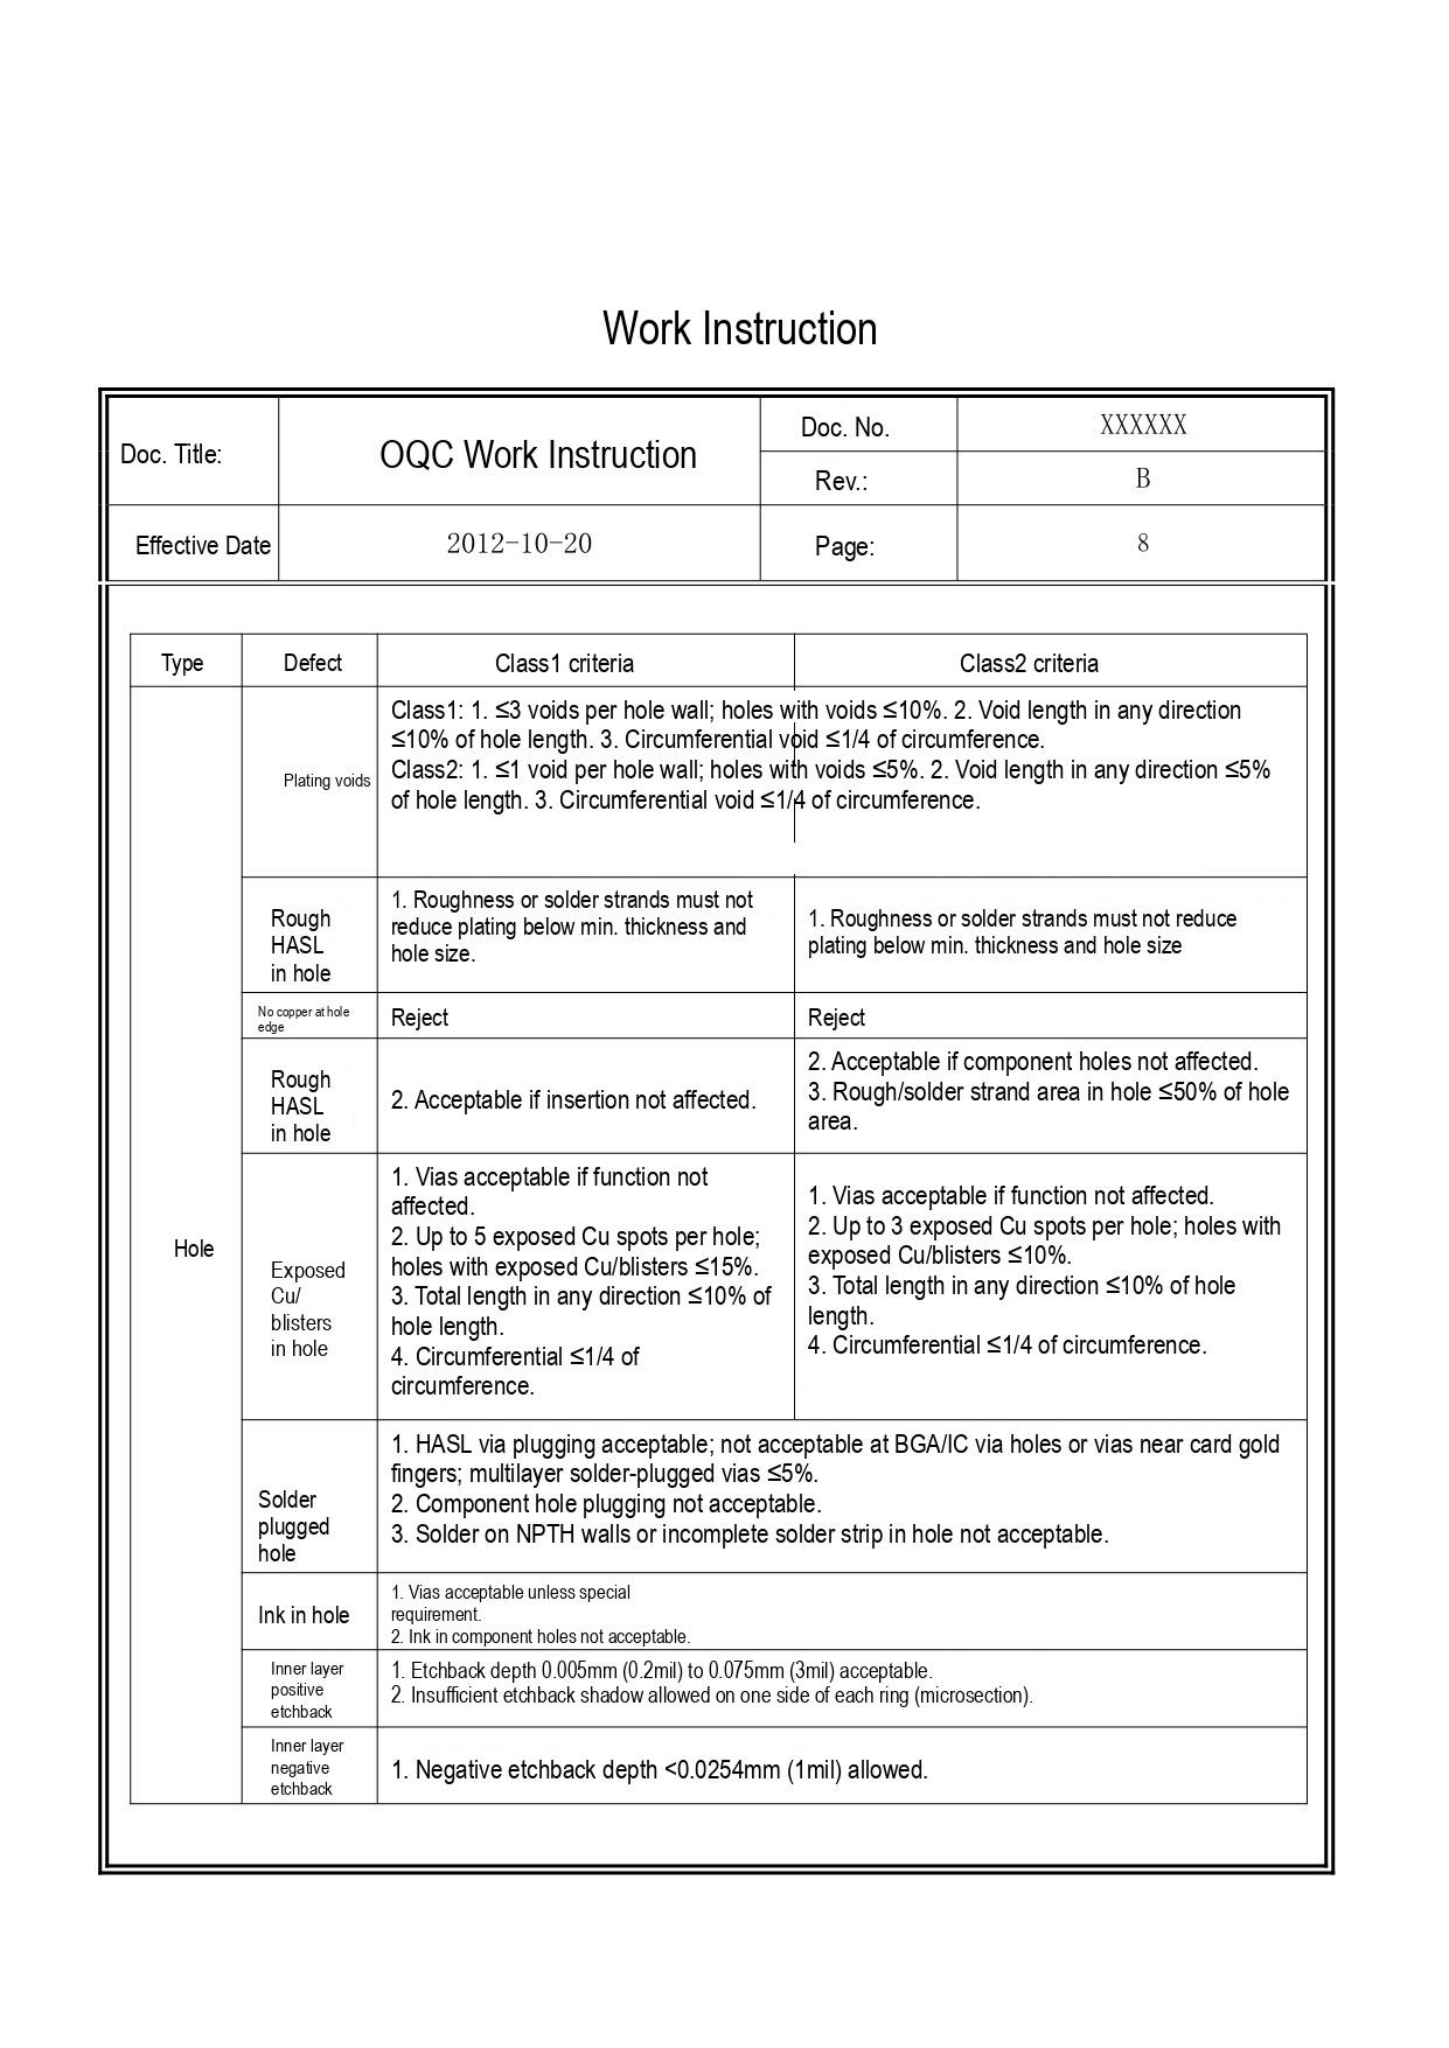# Work Instruction

| Doc. Title: | OQC Work Instruction | Doc. No. | XXXXXX |
|---|---|---|---|
| | | Rev.: | B |
| Effective Date | 2012-10-20 | Page: | 8 |

| Type | Defect | Class1 criteria | Class2 criteria |
|---|---|---|---|
| Hole | Plating voids | Class1: 1. ≤3 voids per hole wall; holes with voids ≤10%. 2. Void length in any direction ≤10% of hole length. 3. Circumferential void ≤1/4 of circumference.<br>Class2: 1. ≤1 void per hole wall; holes with voids ≤5%. 2. Void length in any direction ≤5% of hole length. 3. Circumferential void ≤1/4 of circumference. | |
| | Rough HASL in hole | 1. Roughness or solder strands must not reduce plating below min. thickness and hole size. | 1. Roughness or solder strands must not reduce plating below min. thickness and hole size |
| | No copper at hole edge | Reject | Reject |
| | Rough HASL in hole | 2. Acceptable if insertion not affected. | 2. Acceptable if component holes not affected.<br>3. Rough/solder strand area in hole ≤50% of hole area. |
| | Exposed Cu/ blisters in hole | 1. Vias acceptable if function not affected.<br>2. Up to 5 exposed Cu spots per hole; holes with exposed Cu/blisters ≤15%.<br>3. Total length in any direction ≤10% of hole length.<br>4. Circumferential ≤1/4 of circumference. | 1. Vias acceptable if function not affected.<br>2. Up to 3 exposed Cu spots per hole; holes with exposed Cu/blisters ≤10%.<br>3. Total length in any direction ≤10% of hole length.<br>4. Circumferential ≤1/4 of circumference. |
| | Solder plugged hole | 1. HASL via plugging acceptable; not acceptable at BGA/IC via holes or vias near card gold fingers; multilayer solder-plugged vias ≤5%.<br>2. Component hole plugging not acceptable.<br>3. Solder on NPTH walls or incomplete solder strip in hole not acceptable. | |
| | Ink in hole | 1. Vias acceptable unless special requirement.<br>2. Ink in component holes not acceptable. | |
| | Inner layer positive etchback | 1. Etchback depth 0.005mm (0.2mil) to 0.075mm (3mil) acceptable.<br>2. Insufficient etchback shadow allowed on one side of each ring (microsection). | |
| | Inner layer negative etchback | 1. Negative etchback depth <0.0254mm (1mil) allowed. | |
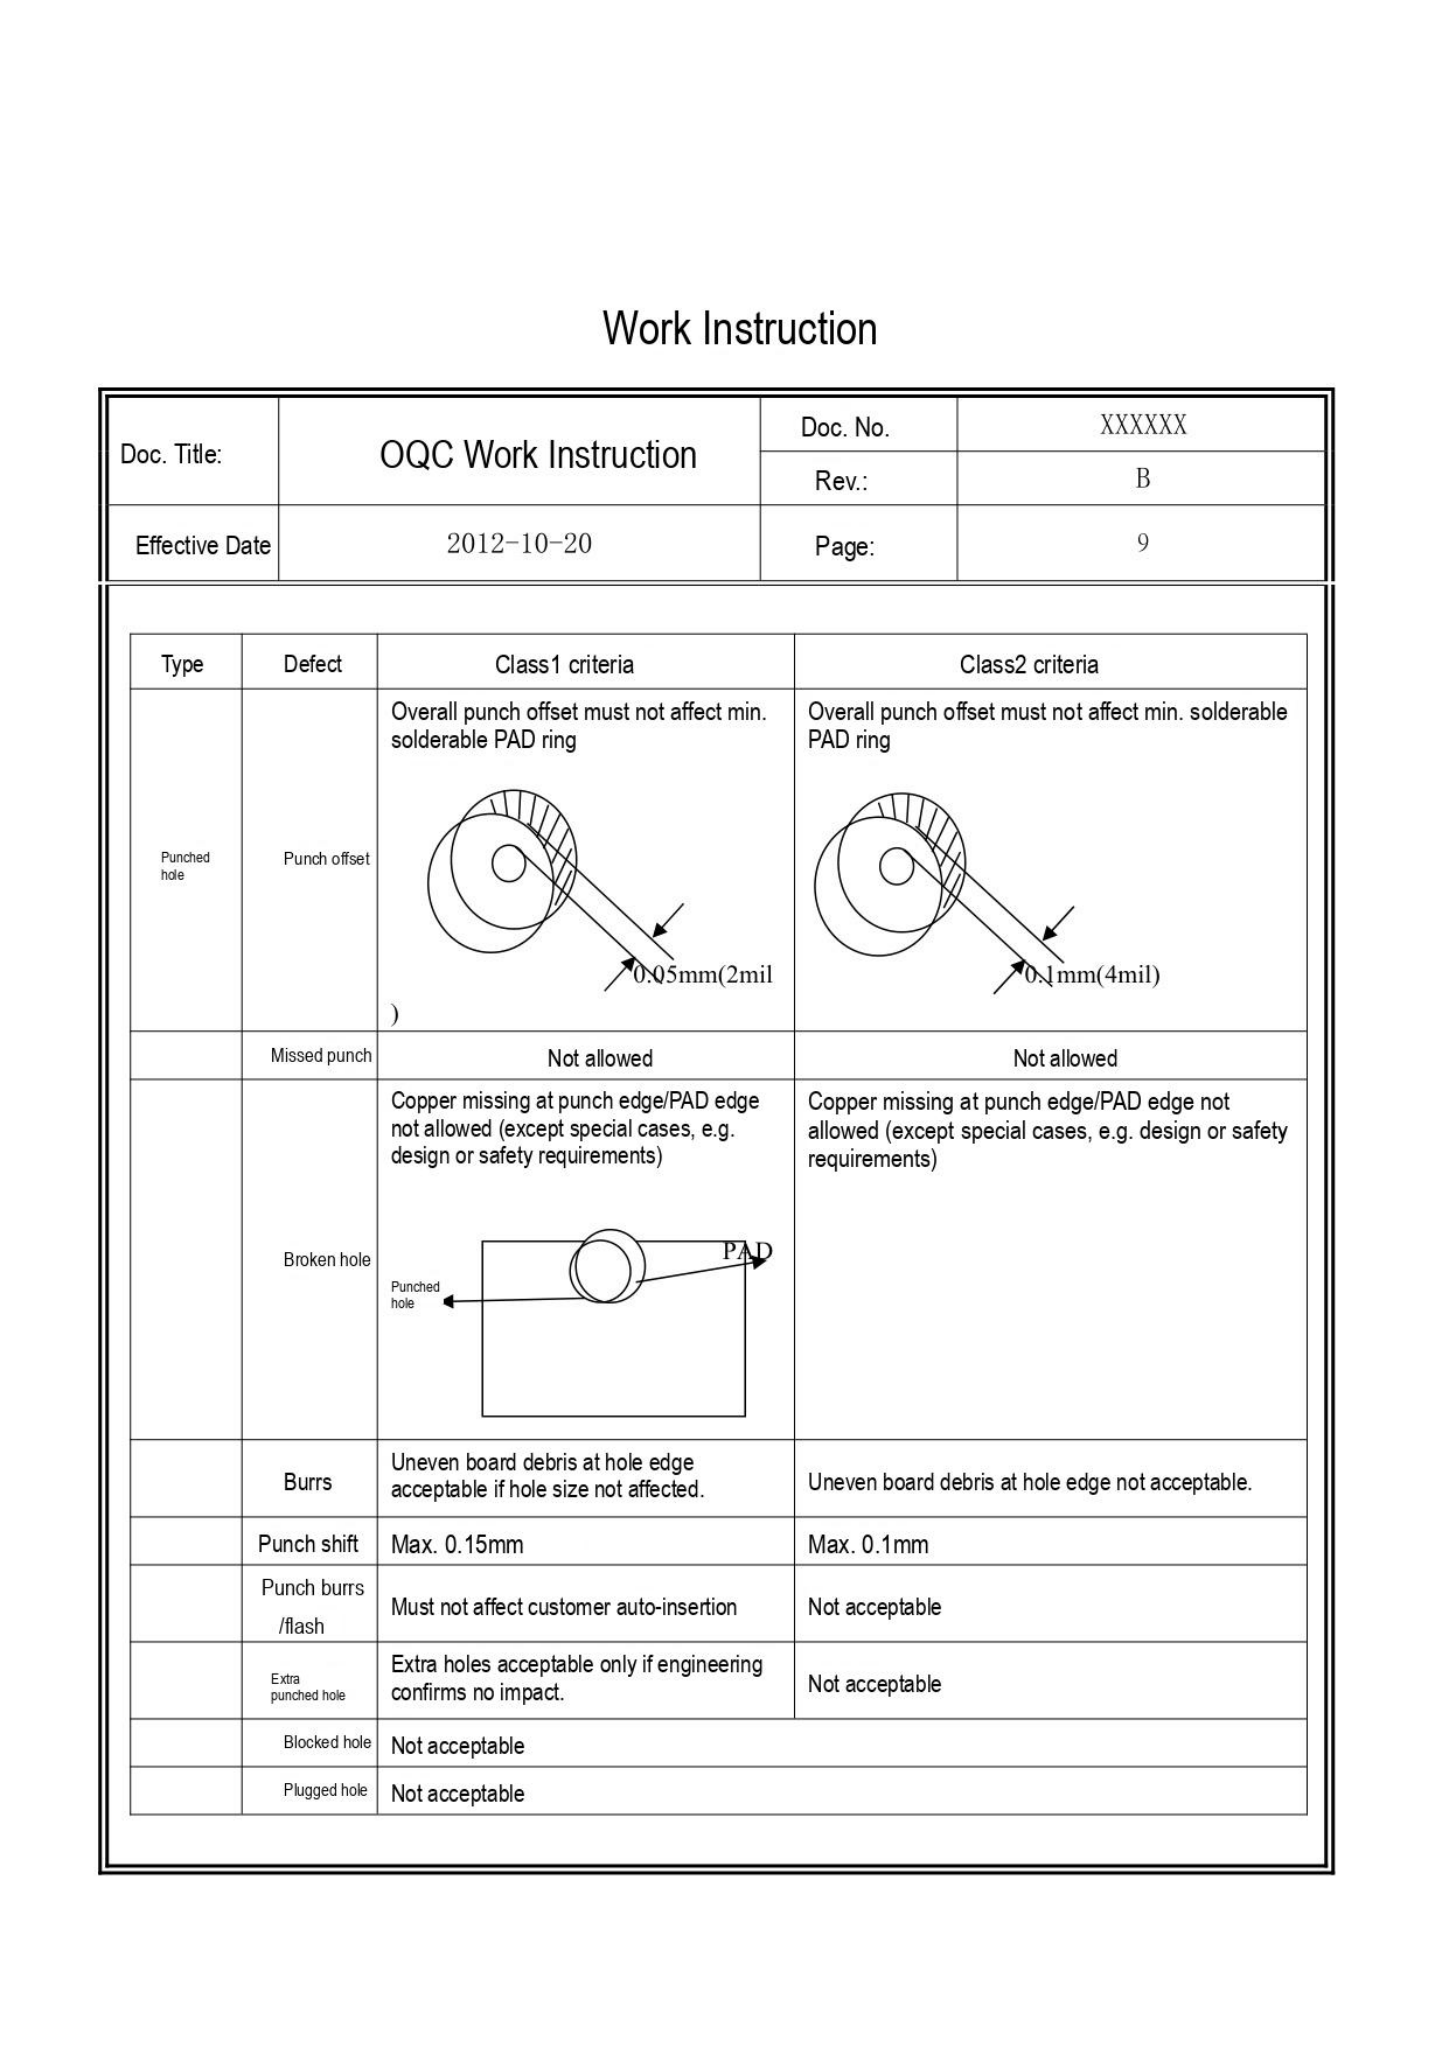Work Instruction

| Doc. Title: | OQC Work Instruction | Doc. No. | XXXXXX |
|---|---|---|---|
| | | Rev.: | B |
| Effective Date | 2012-10-20 | Page: | 9 |

| Type | Defect | Class1 criteria | Class2 criteria |
|---|---|---|---|
| Punched hole | Punch offset | Overall punch offset must not affect min. solderable PAD ring<br>0.05mm(2mil<br>) | Overall punch offset must not affect min. solderable PAD ring<br>0.1mm(4mil) |
| | Missed punch | Not allowed | Not allowed |
| | Broken hole | Copper missing at punch edge/PAD edge not allowed (except special cases, e.g. design or safety requirements)<br>PAD<br>Punched hole | Copper missing at punch edge/PAD edge not allowed (except special cases, e.g. design or safety requirements) |
| | Burrs | Uneven board debris at hole edge acceptable if hole size not affected. | Uneven board debris at hole edge not acceptable. |
| | Punch shift | Max. 0.15mm | Max. 0.1mm |
| | Punch burrs /flash | Must not affect customer auto-insertion | Not acceptable |
| | Extra punched hole | Extra holes acceptable only if engineering confirms no impact. | Not acceptable |
| | Blocked hole | Not acceptable | |
| | Plugged hole | Not acceptable | |
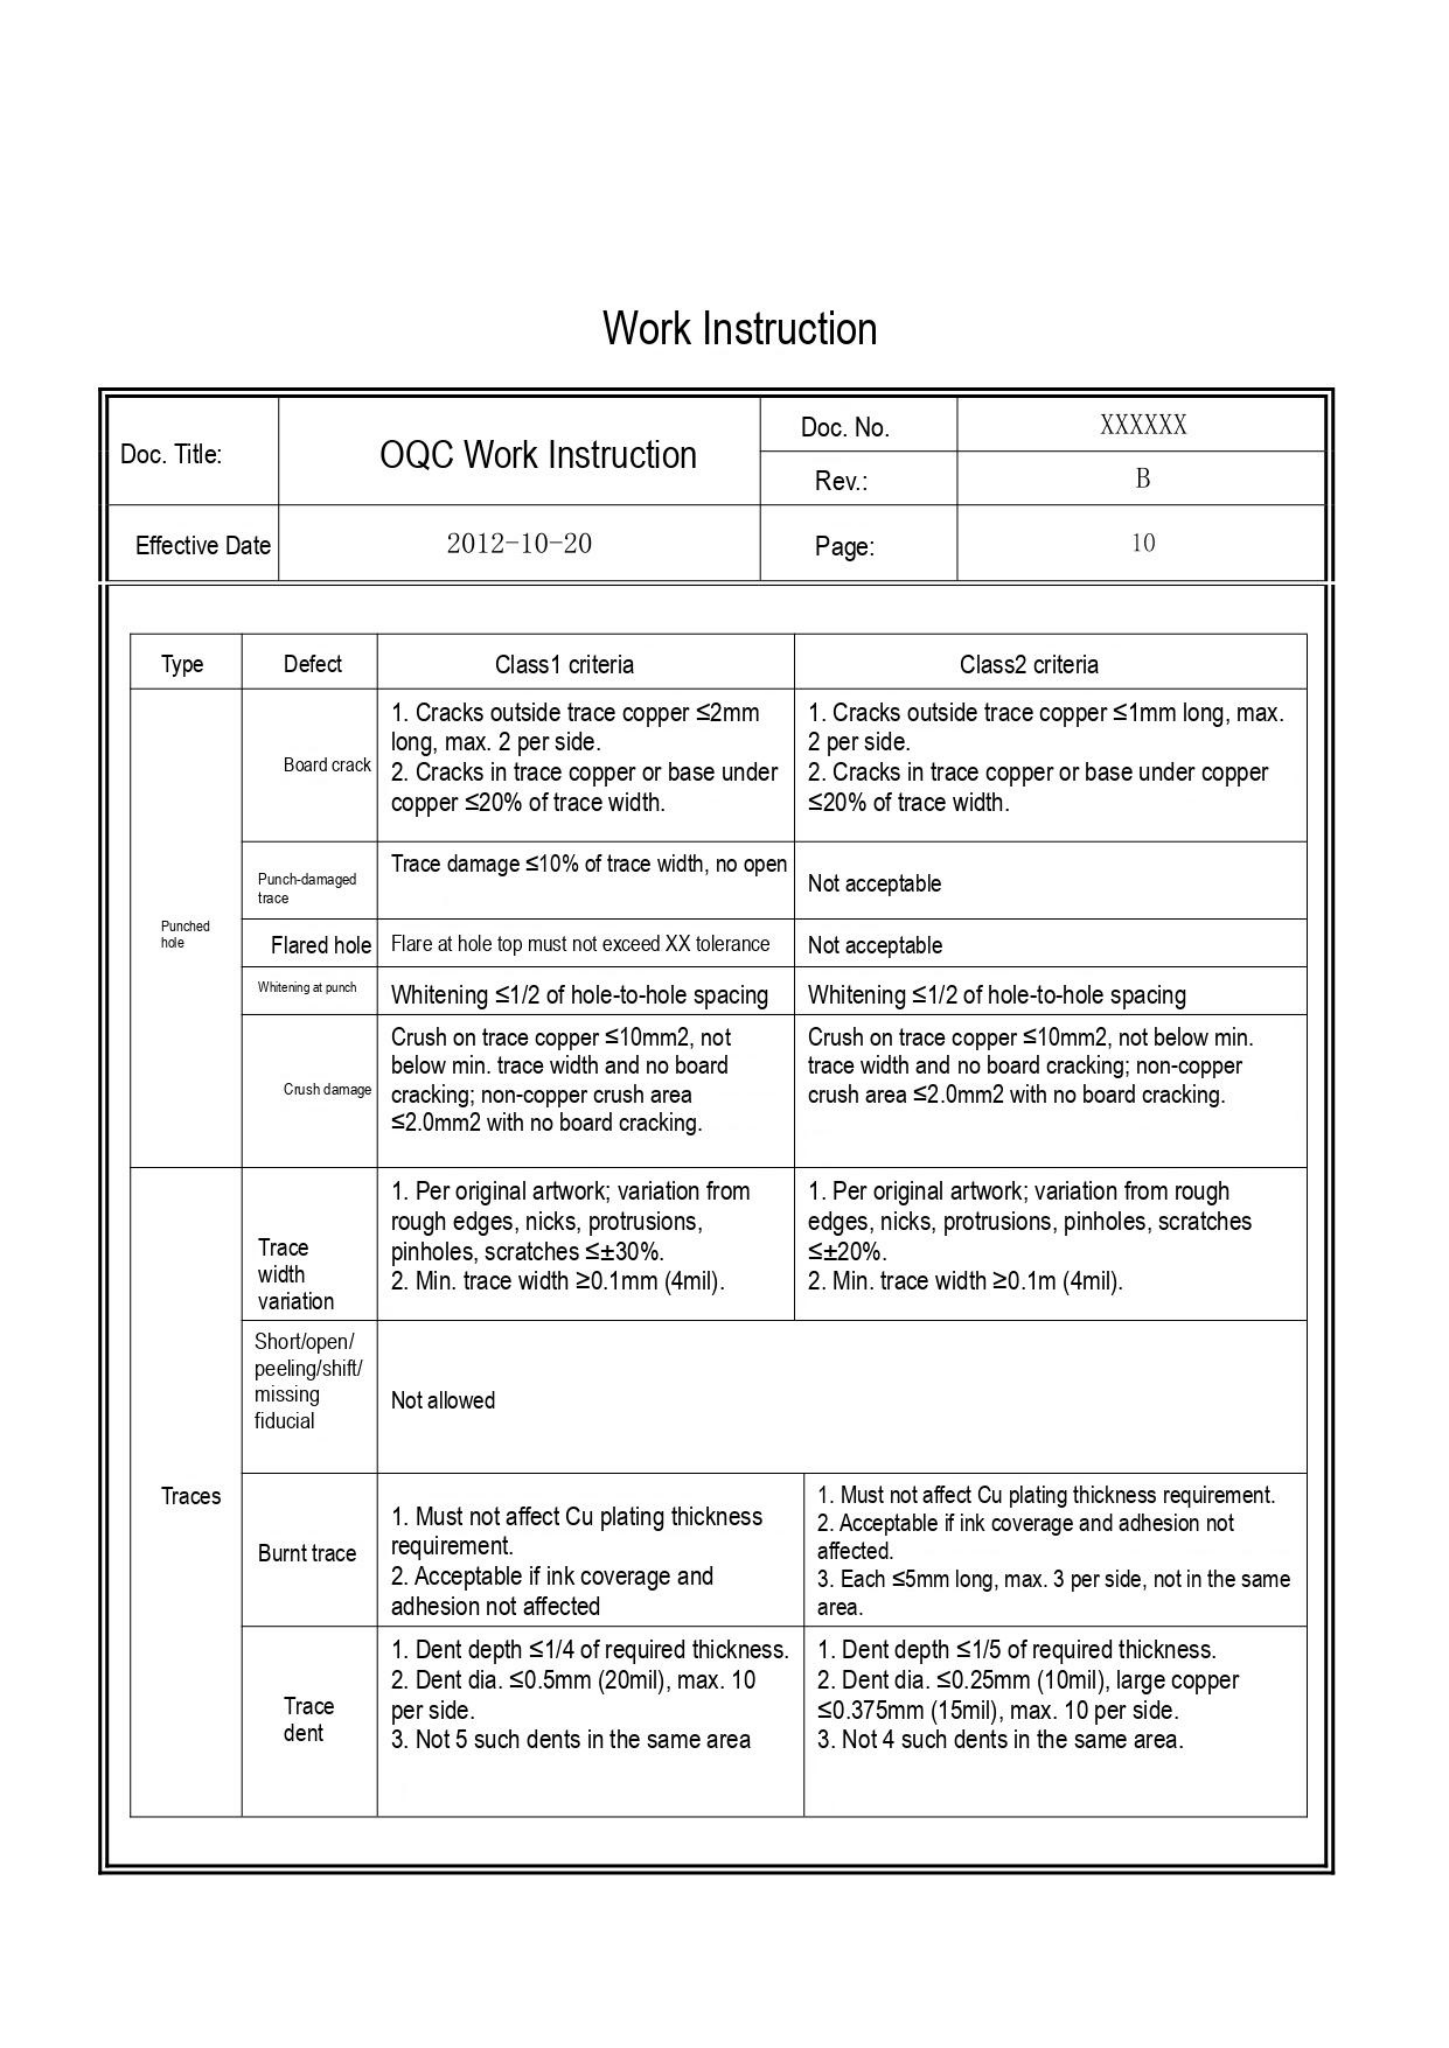Work Instruction

| Doc. Title: | OQC Work Instruction | Doc. No. | XXXXXX |
|---|---|---|---|
| | | Rev.: | B |
| Effective Date | 2012-10-20 | Page: | 10 |

| Type | Defect | Class1 criteria | Class2 criteria |
|---|---|---|---|
| Punched hole | Board crack | 1. Cracks outside trace copper ≤2mm long, max. 2 per side.<br>2. Cracks in trace copper or base under copper ≤20% of trace width. | 1. Cracks outside trace copper ≤1mm long, max. 2 per side.<br>2. Cracks in trace copper or base under copper ≤20% of trace width. |
| Punched hole | Punch-damaged trace | Trace damage ≤10% of trace width, no open | Not acceptable |
| Punched hole | Flared hole | Flare at hole top must not exceed XX tolerance | Not acceptable |
| Punched hole | Whitening at punch | Whitening ≤1/2 of hole-to-hole spacing | Whitening ≤1/2 of hole-to-hole spacing |
| Punched hole | Crush damage | Crush on trace copper ≤10mm2, not below min. trace width and no board cracking; non-copper crush area ≤2.0mm2 with no board cracking. | Crush on trace copper ≤10mm2, not below min. trace width and no board cracking; non-copper crush area ≤2.0mm2 with no board cracking. |
| Traces | Trace width variation | 1. Per original artwork; variation from rough edges, nicks, protrusions, pinholes, scratches ≤±30%.<br>2. Min. trace width ≥0.1mm (4mil). | 1. Per original artwork; variation from rough edges, nicks, protrusions, pinholes, scratches ≤±20%.<br>2. Min. trace width ≥0.1m (4mil). |
| Traces | Short/open/ peeling/shift/ missing fiducial | Not allowed | Not allowed |
| Traces | Burnt trace | 1. Must not affect Cu plating thickness requirement.<br>2. Acceptable if ink coverage and adhesion not affected | 1. Must not affect Cu plating thickness requirement.<br>2. Acceptable if ink coverage and adhesion not affected.<br>3. Each ≤5mm long, max. 3 per side, not in the same area. |
| Traces | Trace dent | 1. Dent depth ≤1/4 of required thickness.<br>2. Dent dia. ≤0.5mm (20mil), max. 10 per side.<br>3. Not 5 such dents in the same area | 1. Dent depth ≤1/5 of required thickness.<br>2. Dent dia. ≤0.25mm (10mil), large copper ≤0.375mm (15mil), max. 10 per side.<br>3. Not 4 such dents in the same area. |
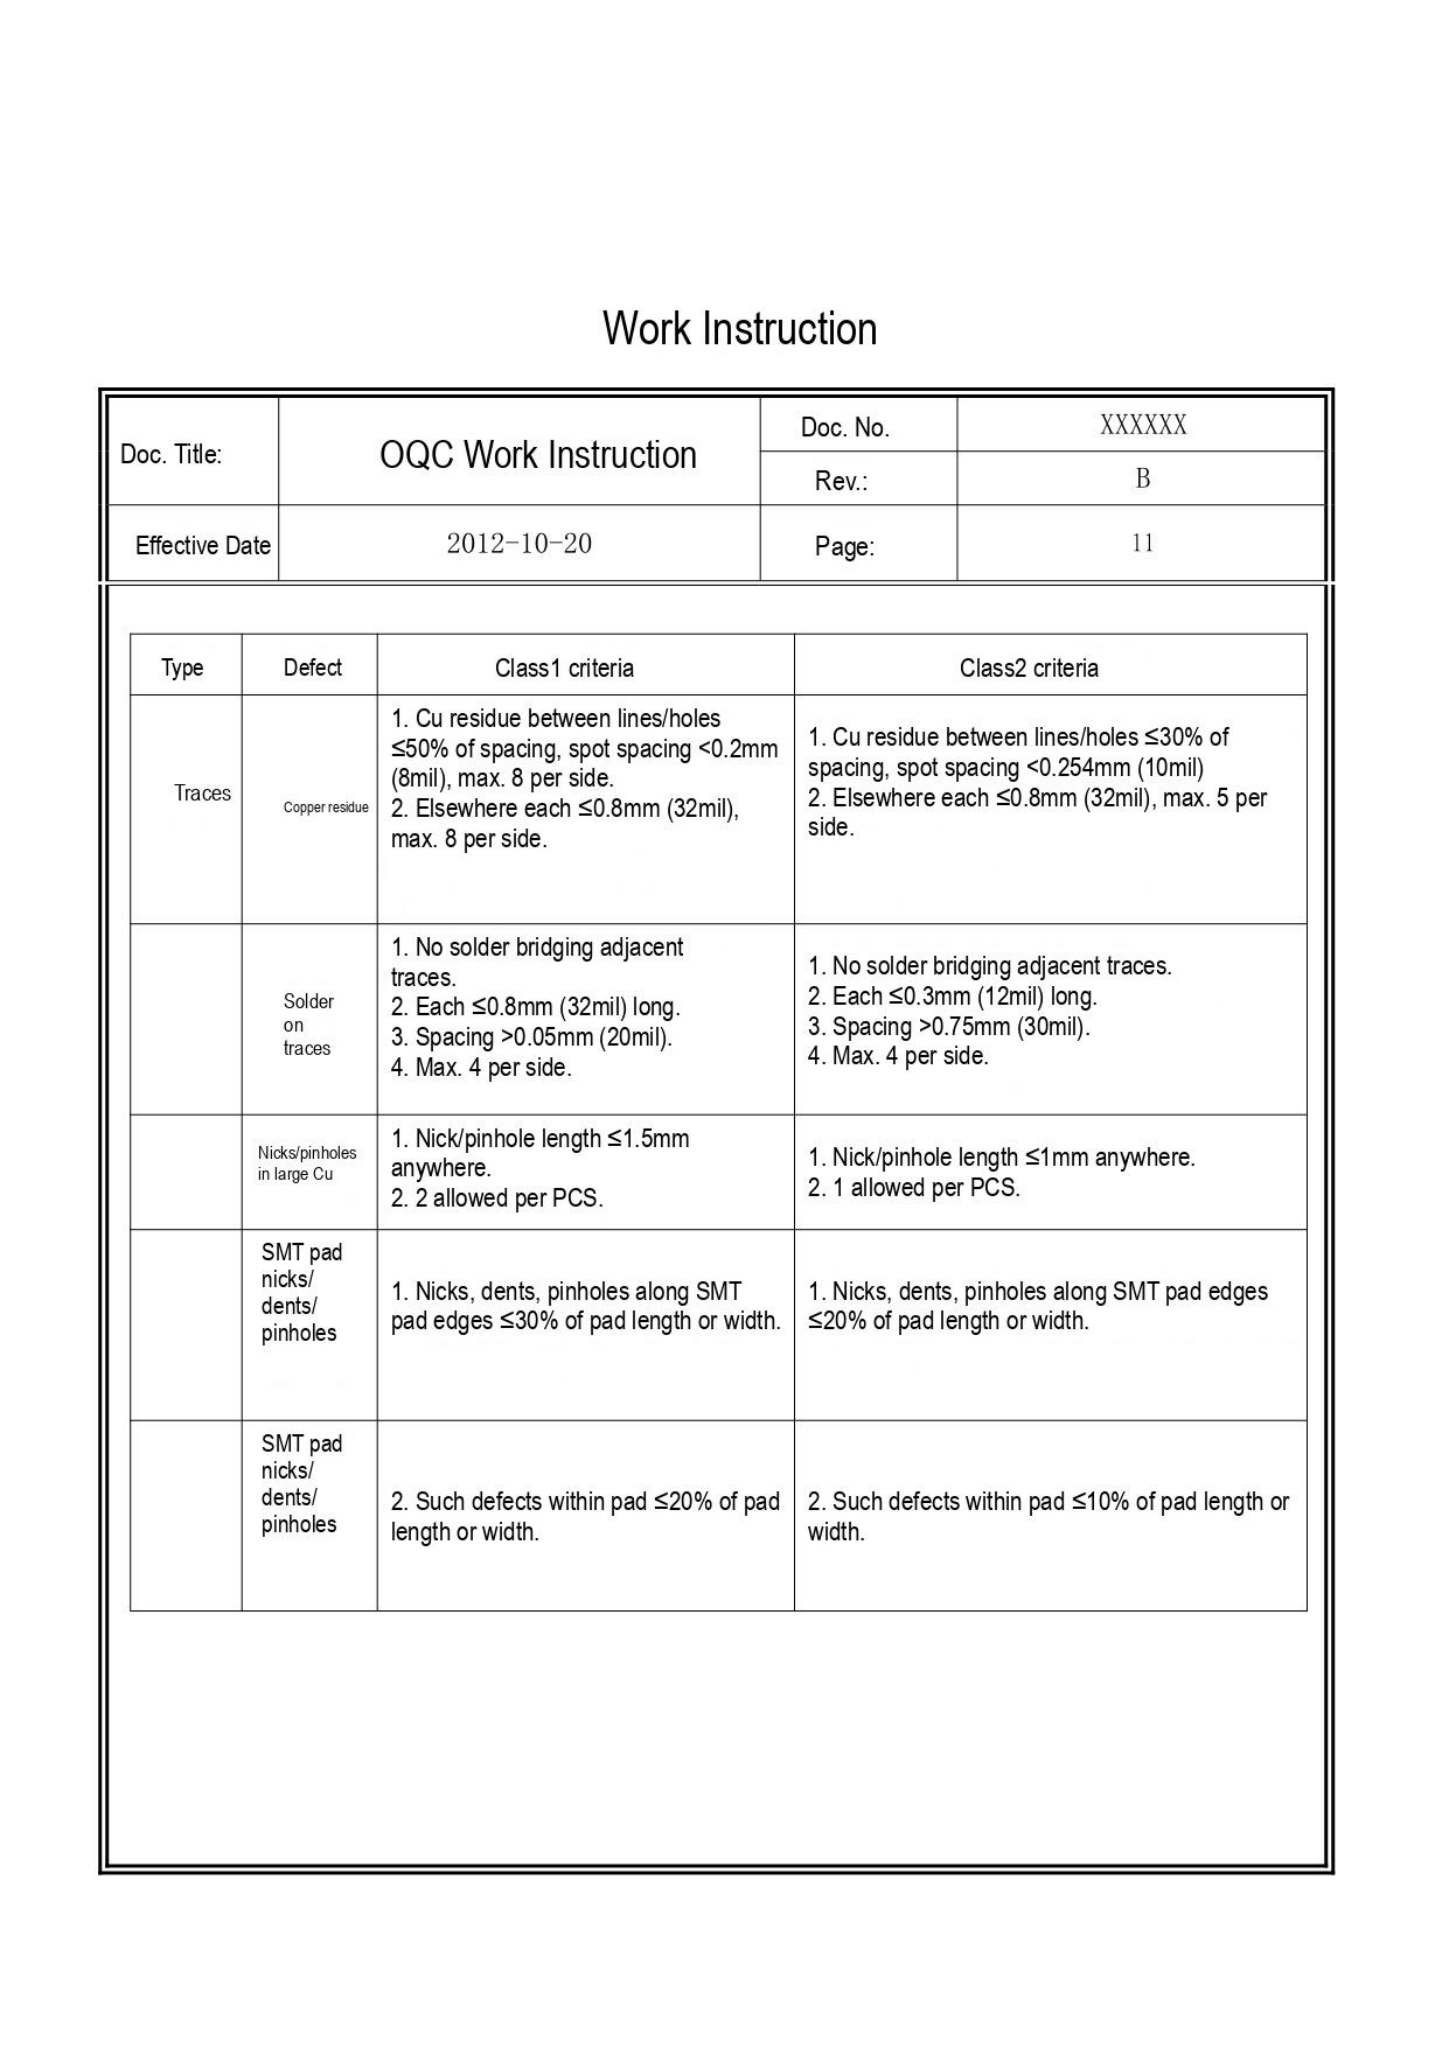Work Instruction

| Doc. Title: | OQC Work Instruction | Doc. No. | XXXXXX |
|---|---|---|---|
| | | Rev.: | B |
| Effective Date | 2012-10-20 | Page: | 11 |

| Type | Defect | Class1 criteria | Class2 criteria |
|---|---|---|---|
| Traces | Copper residue | 1. Cu residue between lines/holes ≤50% of spacing, spot spacing <0.2mm (8mil), max. 8 per side.<br>2. Elsewhere each ≤0.8mm (32mil), max. 8 per side. | 1. Cu residue between lines/holes ≤30% of spacing, spot spacing <0.254mm (10mil)<br>2. Elsewhere each ≤0.8mm (32mil), max. 5 per side. |
| | Solder on traces | 1. No solder bridging adjacent traces.<br>2. Each ≤0.8mm (32mil) long.<br>3. Spacing >0.05mm (20mil).<br>4. Max. 4 per side. | 1. No solder bridging adjacent traces.<br>2. Each ≤0.3mm (12mil) long.<br>3. Spacing >0.75mm (30mil).<br>4. Max. 4 per side. |
| | Nicks/pinholes in large Cu | 1. Nick/pinhole length ≤1.5mm anywhere.<br>2. 2 allowed per PCS. | 1. Nick/pinhole length ≤1mm anywhere.<br>2. 1 allowed per PCS. |
| | SMT pad nicks/ dents/ pinholes | 1. Nicks, dents, pinholes along SMT pad edges ≤30% of pad length or width. | 1. Nicks, dents, pinholes along SMT pad edges ≤20% of pad length or width. |
| | SMT pad nicks/ dents/ pinholes | 2. Such defects within pad ≤20% of pad length or width. | 2. Such defects within pad ≤10% of pad length or width. |
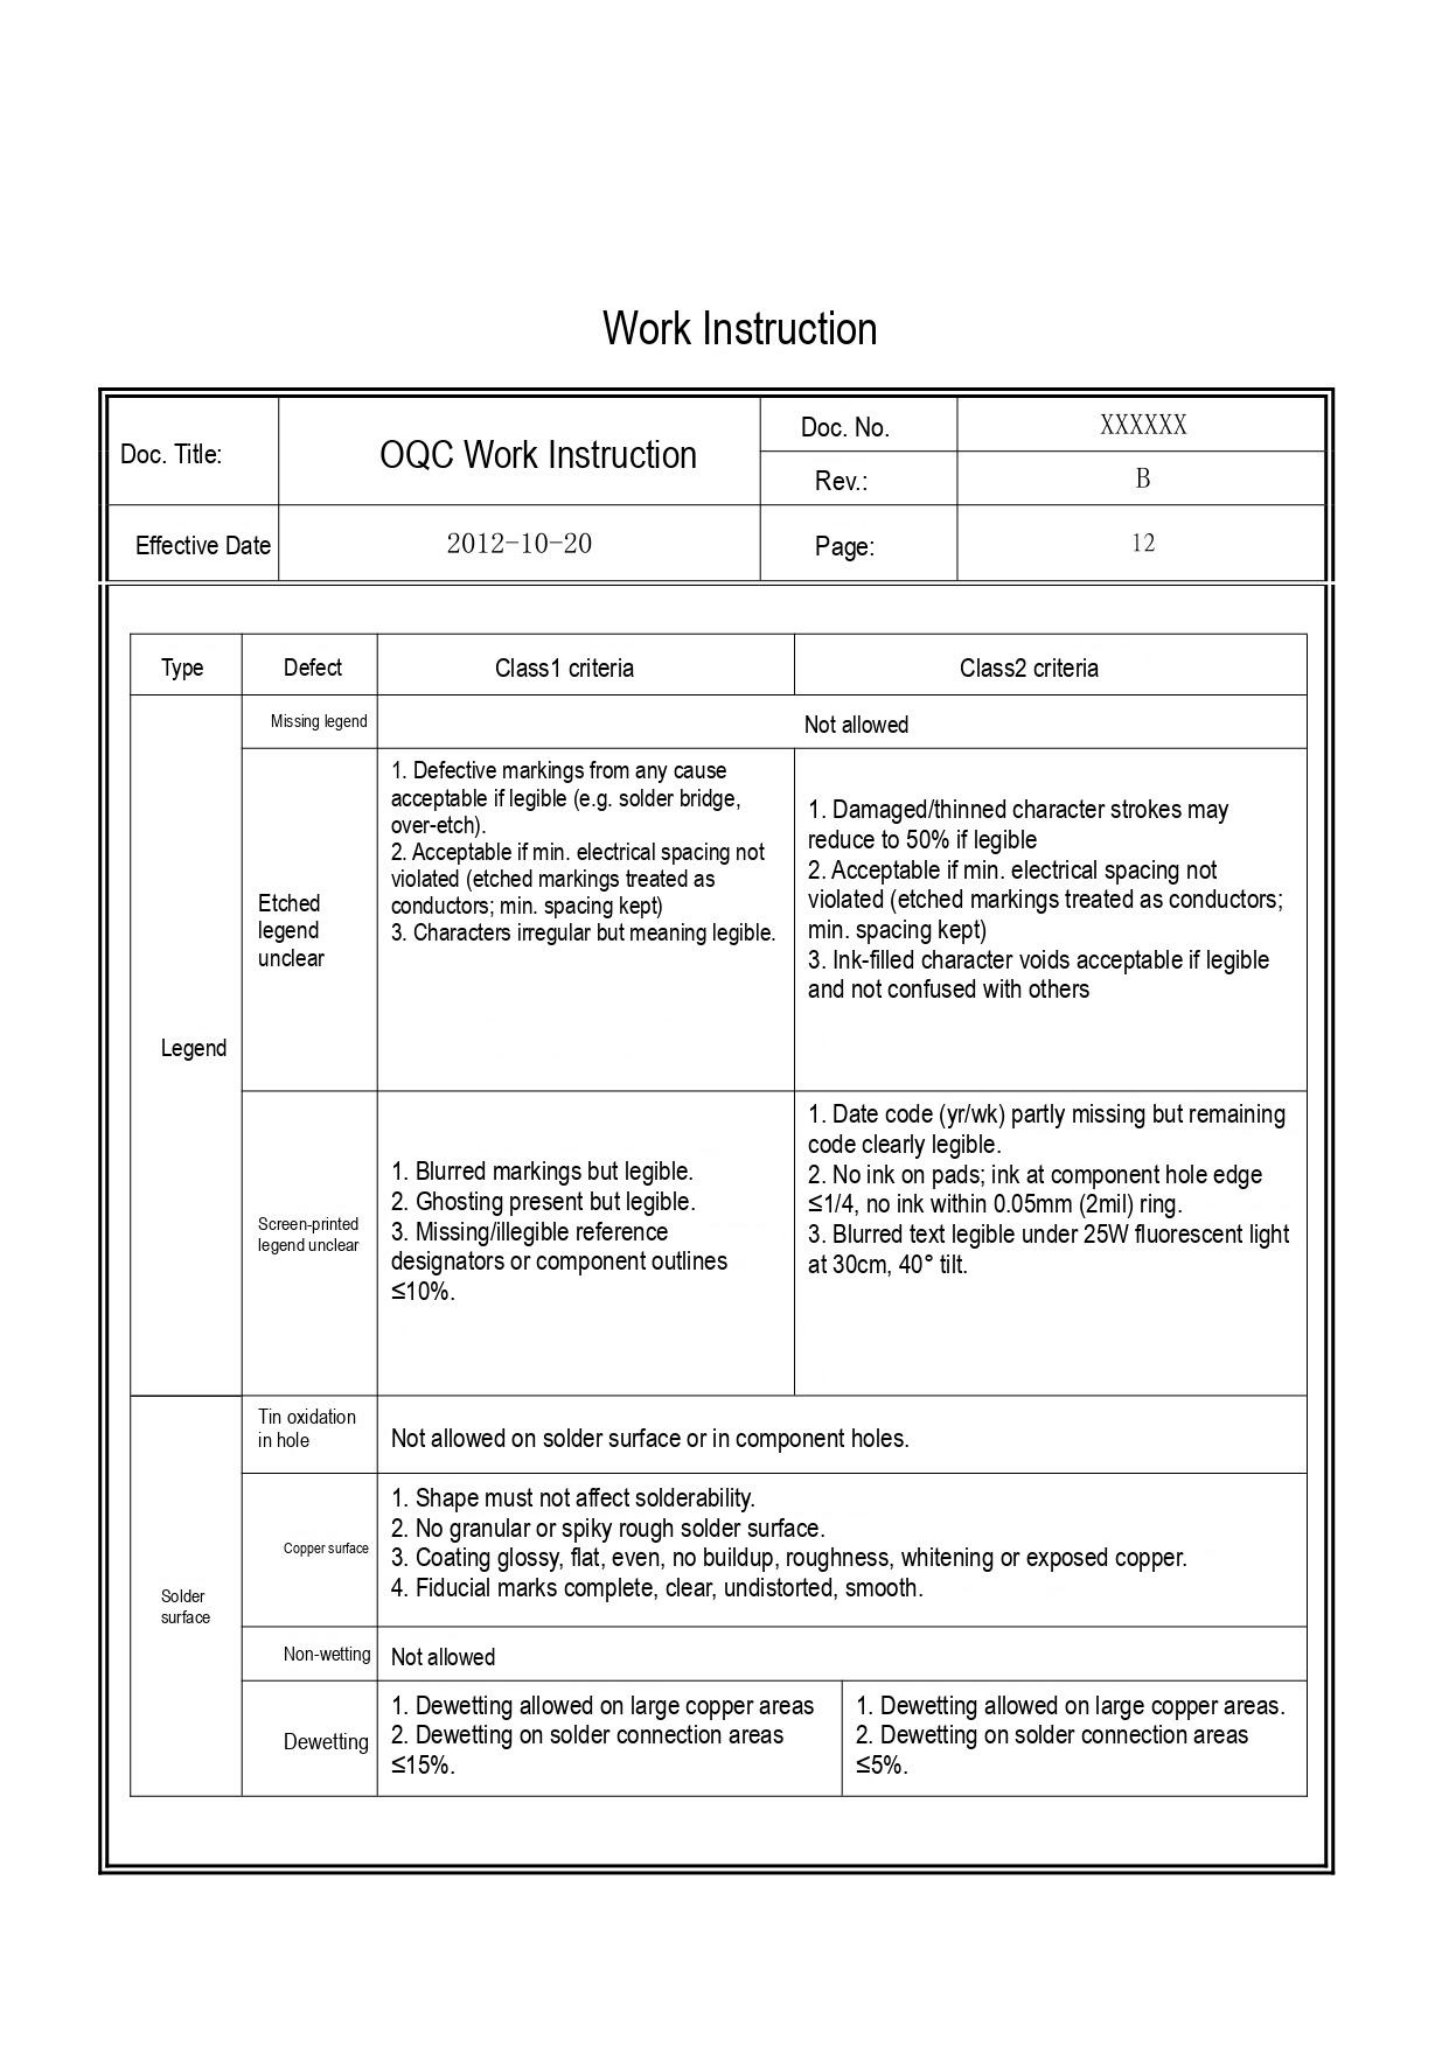Work Instruction

| Doc. Title: | OQC Work Instruction | Doc. No. | XXXXXX |
|---|---|---|---|
| | | Rev.: | B |
| Effective Date | 2012-10-20 | Page: | 12 |

| Type | Defect | Class1 criteria | Class2 criteria |
|---|---|---|---|
| Legend | Missing legend | Not allowed | Not allowed |
| | Etched legend unclear | 1. Defective markings from any cause acceptable if legible (e.g. solder bridge, over-etch).<br>2. Acceptable if min. electrical spacing not violated (etched markings treated as conductors; min. spacing kept)<br>3. Characters irregular but meaning legible. | 1. Damaged/thinned character strokes may reduce to 50% if legible<br>2. Acceptable if min. electrical spacing not violated (etched markings treated as conductors; min. spacing kept)<br>3. Ink-filled character voids acceptable if legible and not confused with others |
| | Screen-printed legend unclear | 1. Blurred markings but legible.<br>2. Ghosting present but legible.<br>3. Missing/illegible reference designators or component outlines ≤10%. | 1. Date code (yr/wk) partly missing but remaining code clearly legible.<br>2. No ink on pads; ink at component hole edge ≤1/4, no ink within 0.05mm (2mil) ring.<br>3. Blurred text legible under 25W fluorescent light at 30cm, 40° tilt. |
| Solder surface | Tin oxidation in hole | Not allowed on solder surface or in component holes. | Not allowed on solder surface or in component holes. |
| | Copper surface | 1. Shape must not affect solderability.<br>2. No granular or spiky rough solder surface.<br>3. Coating glossy, flat, even, no buildup, roughness, whitening or exposed copper.<br>4. Fiducial marks complete, clear, undistorted, smooth. | 1. Shape must not affect solderability.<br>2. No granular or spiky rough solder surface.<br>3. Coating glossy, flat, even, no buildup, roughness, whitening or exposed copper.<br>4. Fiducial marks complete, clear, undistorted, smooth. |
| | Non-wetting | Not allowed | Not allowed |
| | Dewetting | 1. Dewetting allowed on large copper areas<br>2. Dewetting on solder connection areas ≤15%. | 1. Dewetting allowed on large copper areas.<br>2. Dewetting on solder connection areas ≤5%. |
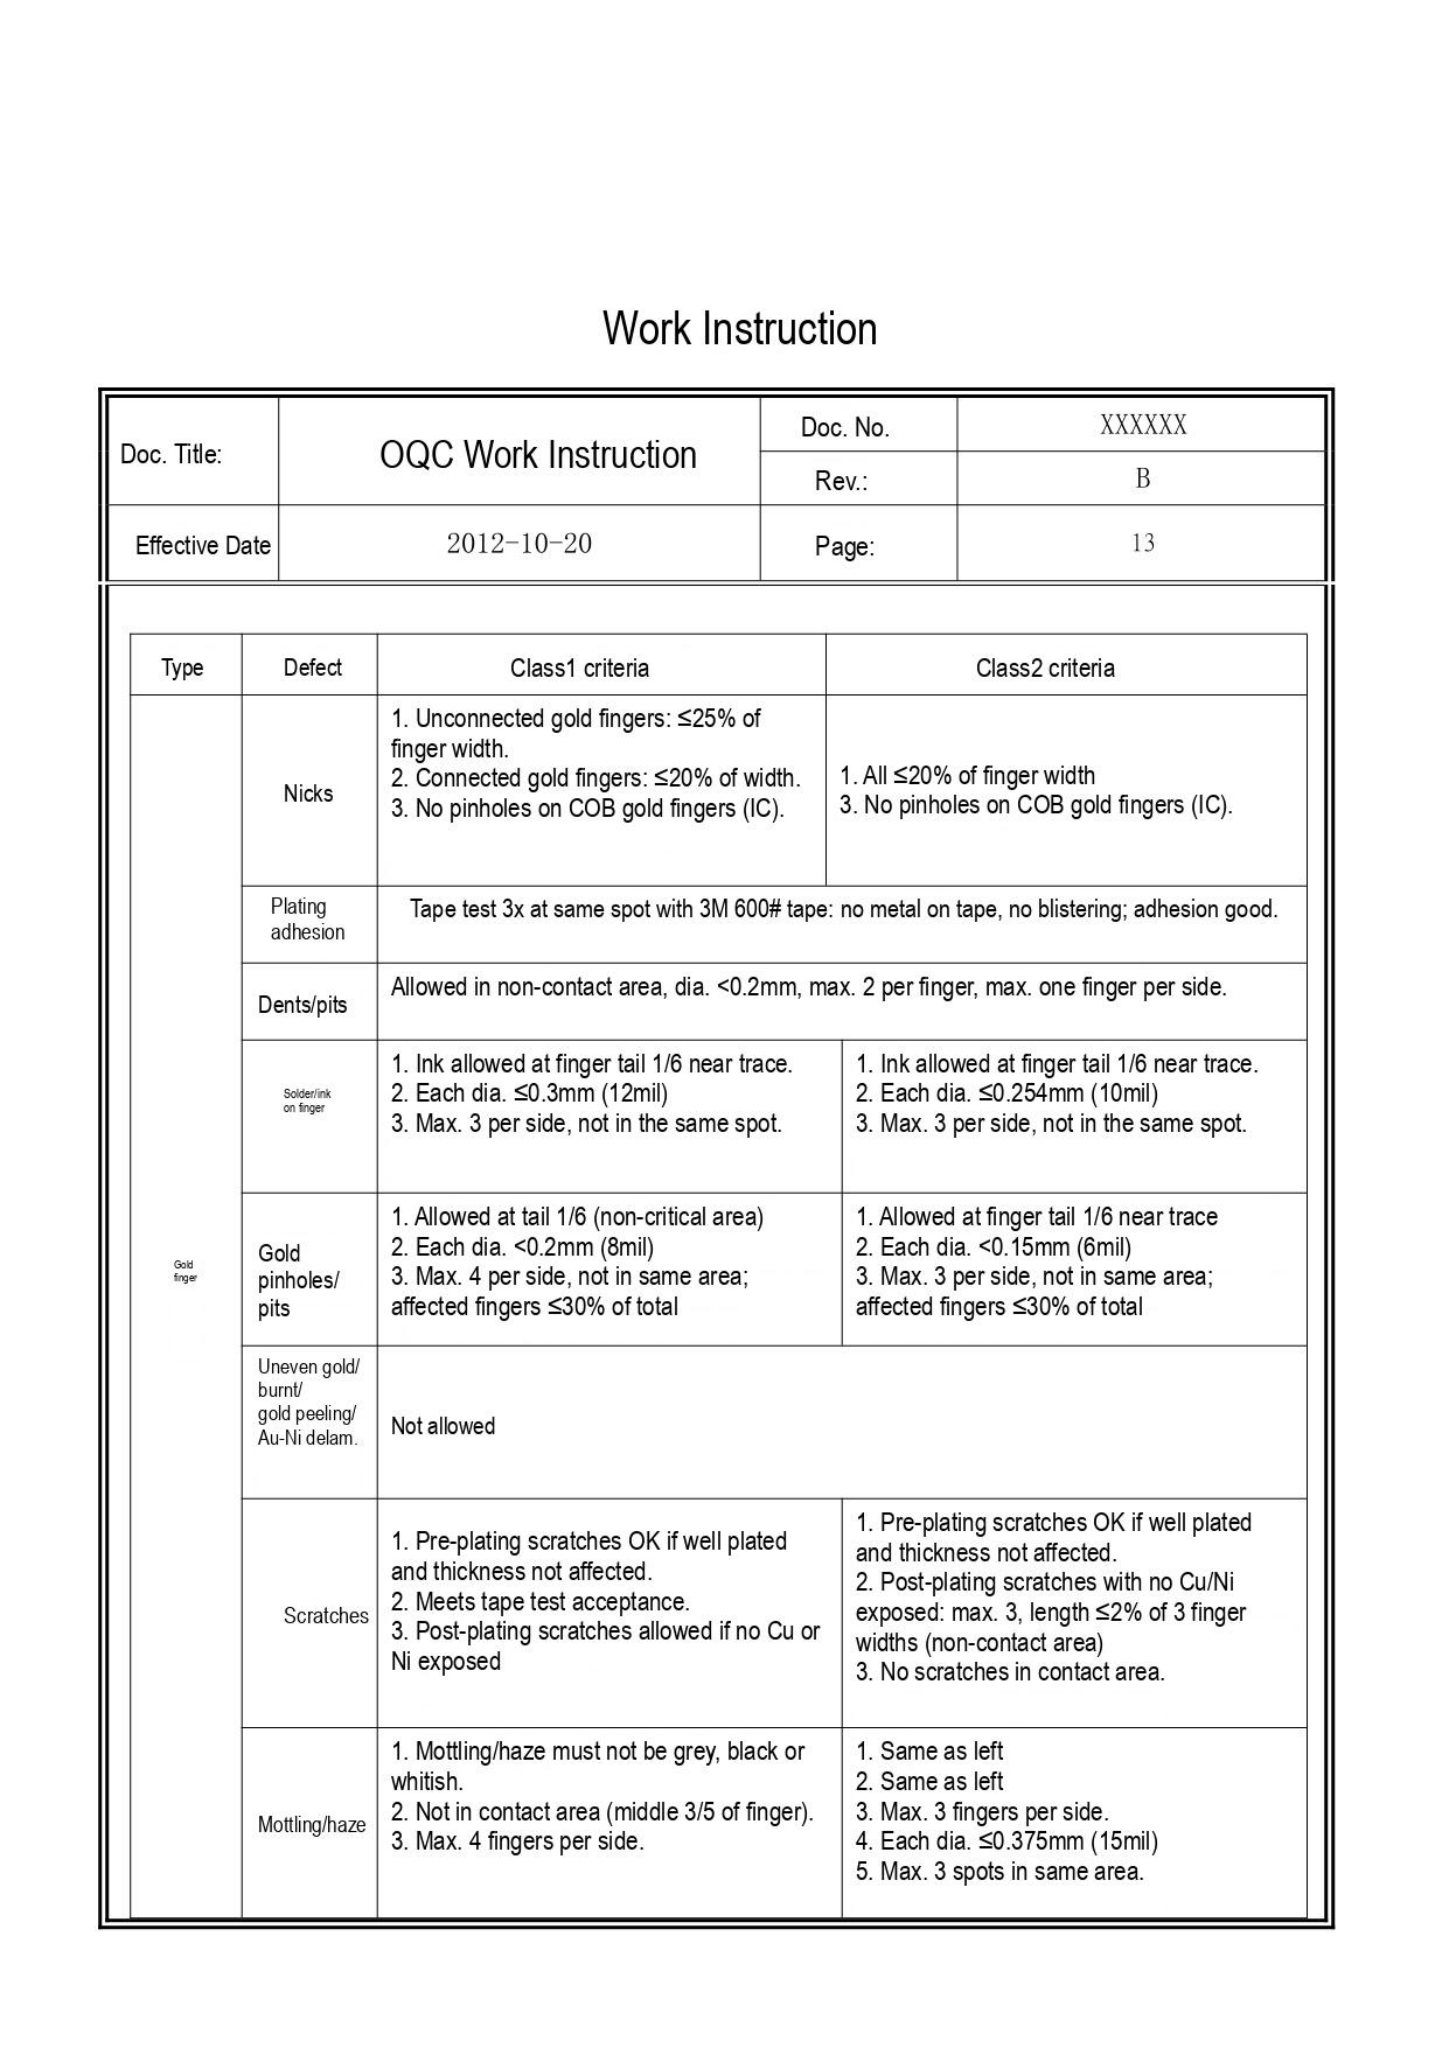Work Instruction

| Doc. Title: | OQC Work Instruction | Doc. No. | XXXXXX |
|---|---|---|---|
| | | Rev.: | B |
| Effective Date | 2012-10-20 | Page: | 13 |

| Type | Defect | Class1 criteria | Class2 criteria |
|---|---|---|---|
| Gold finger | Nicks | 1. Unconnected gold fingers: ≤25% of finger width.<br>2. Connected gold fingers: ≤20% of width.<br>3. No pinholes on COB gold fingers (IC). | 1. All ≤20% of finger width<br>3. No pinholes on COB gold fingers (IC). |
| | Plating adhesion | Tape test 3x at same spot with 3M 600# tape: no metal on tape, no blistering; adhesion good. | |
| | Dents/pits | Allowed in non-contact area, dia. <0.2mm, max. 2 per finger, max. one finger per side. | |
| | Solder/ink on finger | 1. Ink allowed at finger tail 1/6 near trace.<br>2. Each dia. ≤0.3mm (12mil)<br>3. Max. 3 per side, not in the same spot. | 1. Ink allowed at finger tail 1/6 near trace.<br>2. Each dia. ≤0.254mm (10mil)<br>3. Max. 3 per side, not in the same spot. |
| | Gold pinholes/ pits | 1. Allowed at tail 1/6 (non-critical area)<br>2. Each dia. <0.2mm (8mil)<br>3. Max. 4 per side, not in same area; affected fingers ≤30% of total | 1. Allowed at finger tail 1/6 near trace<br>2. Each dia. <0.15mm (6mil)<br>3. Max. 3 per side, not in same area; affected fingers ≤30% of total |
| | Uneven gold/ burnt/ gold peeling/ Au-Ni delam. | Not allowed | |
| | Scratches | 1. Pre-plating scratches OK if well plated and thickness not affected.<br>2. Meets tape test acceptance.<br>3. Post-plating scratches allowed if no Cu or Ni exposed | 1. Pre-plating scratches OK if well plated and thickness not affected.<br>2. Post-plating scratches with no Cu/Ni exposed: max. 3, length ≤2% of 3 finger widths (non-contact area)<br>3. No scratches in contact area. |
| | Mottling/haze | 1. Mottling/haze must not be grey, black or whitish.<br>2. Not in contact area (middle 3/5 of finger).<br>3. Max. 4 fingers per side. | 1. Same as left<br>2. Same as left<br>3. Max. 3 fingers per side.<br>4. Each dia. ≤0.375mm (15mil)<br>5. Max. 3 spots in same area. |